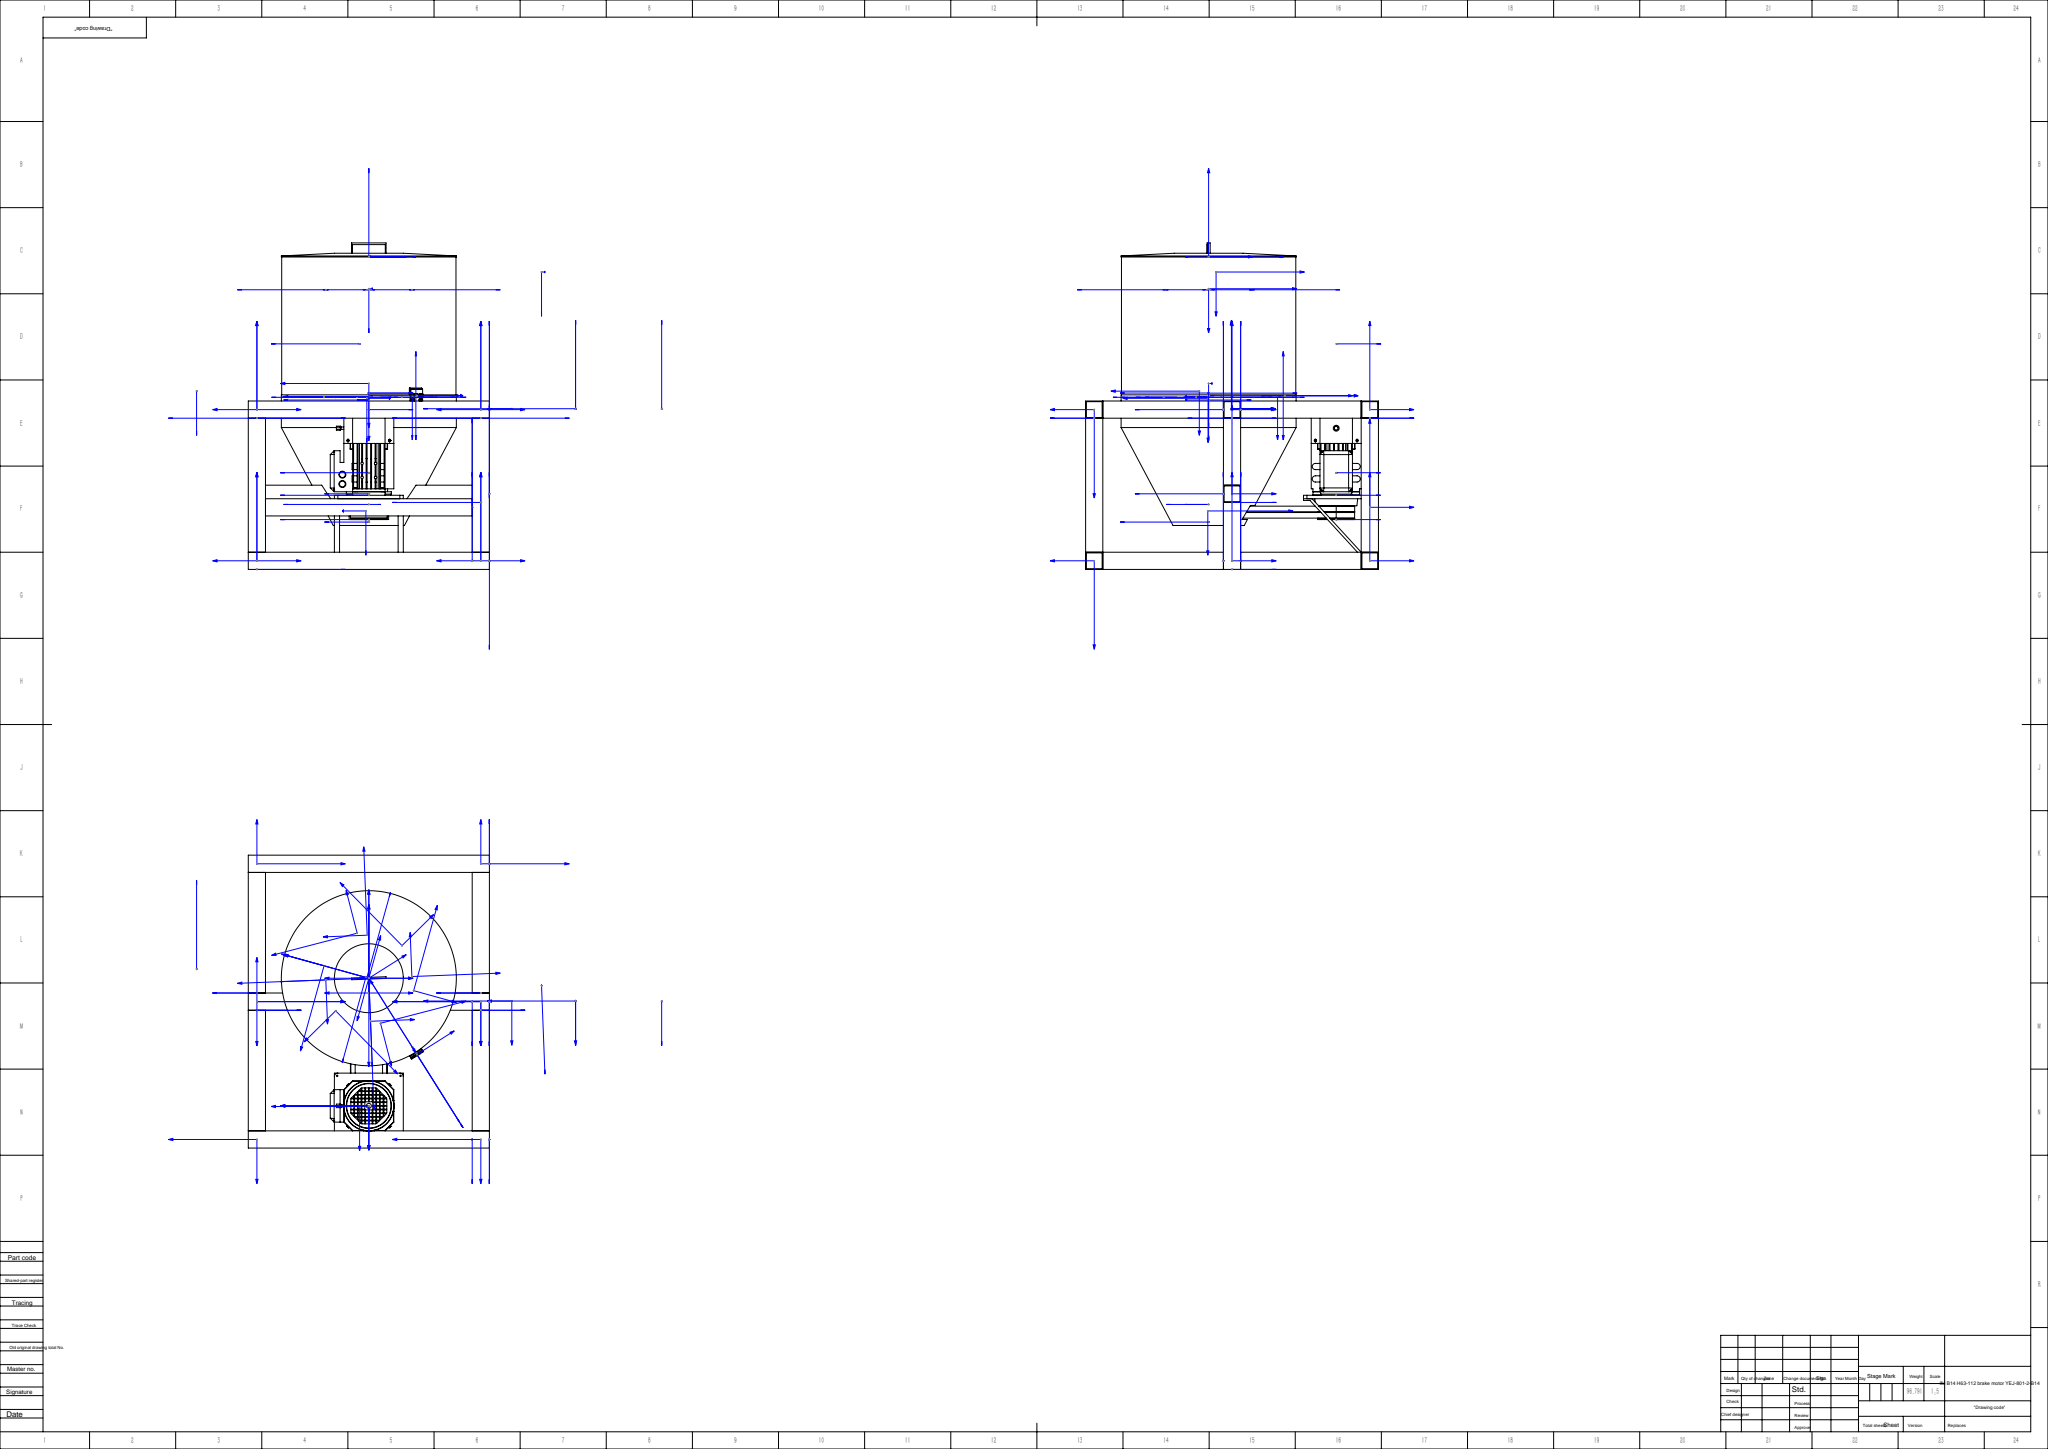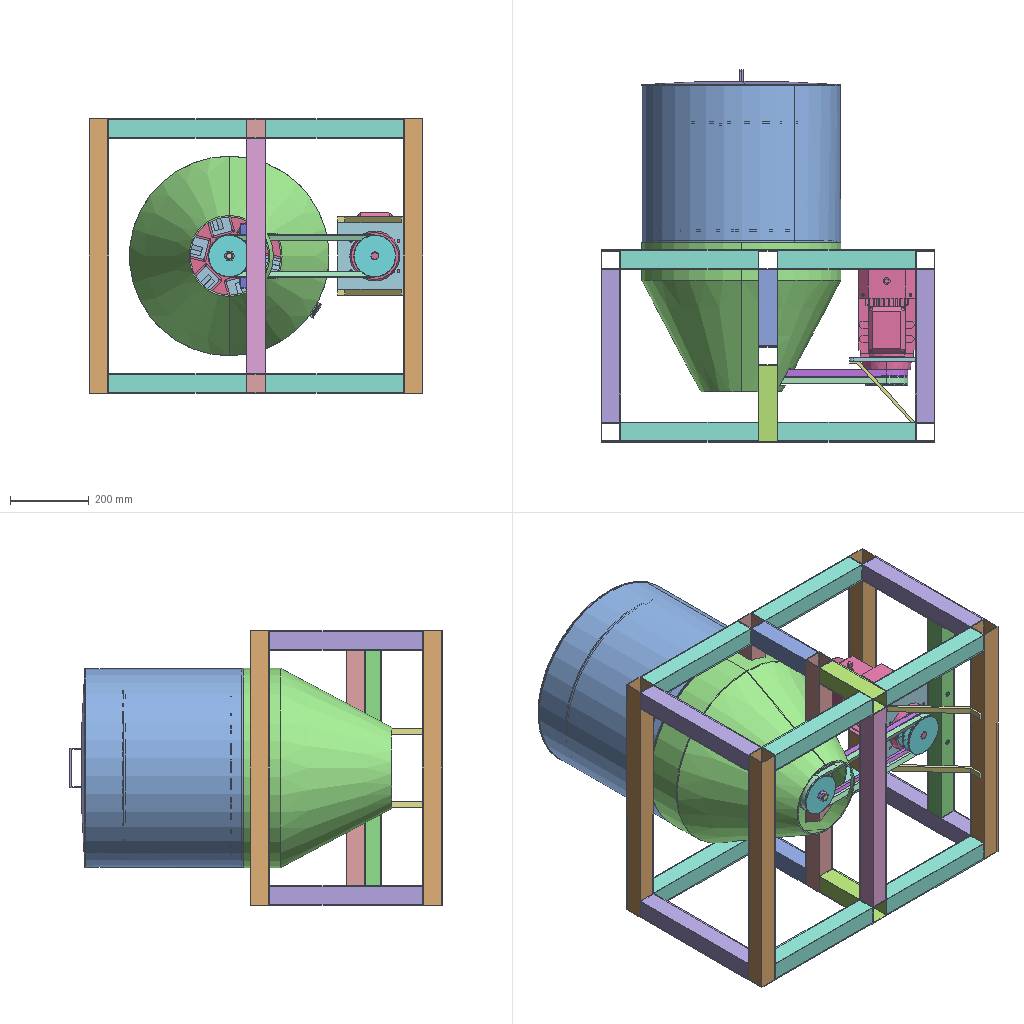Assembly | SolidWorks | 37 different items | 64 placed | box 850 x 948 x 700 mm
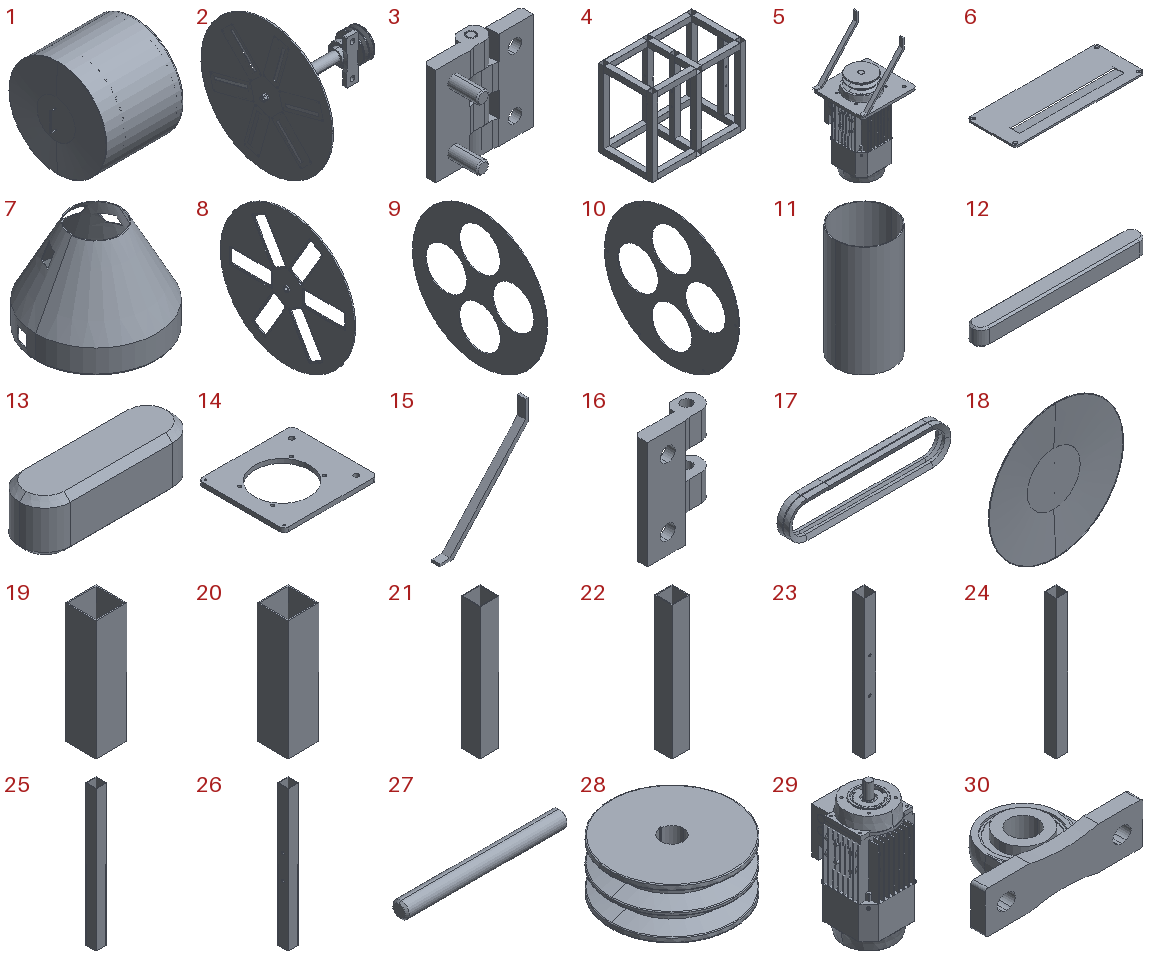Parts list (item | name | quantity | parent item | size | volume | features):
1 | (subassembly) | x1 | - | 463.5 x 508 x 508 mm | 4178464 mm3 | features ReferencePattern 3, LocalCirPattern 1
2 | (subassembly) | x1 | - | 394 x 496 x 496 mm | 1816231 mm3 | features ReferencePattern 5, LocalCirPattern 1
3 | (subassembly) | x1 | in 1 | 40 x 21 x 40 mm | 8853 mm3 | features AEMSimFeature 1
4 | (subassembly) | x1 | - | 850 x 488.8 x 700 mm | 4041372 mm3 | -
5 | (subassembly) | x1 | - | 217.5 x 212 x 474.6 mm | 5596236 mm3 | features CompositeCurve 1, MirrorCompFeat 1, ReferencePattern 1
6 | - | x6 | in 2 | 160 x 60 x 2 mm | 16130 mm3 | features ICE 2, Extrusion 1, Fillet 1, HoleWzd 1
7 | - | x1 | - | 508 x 508 x 384 mm | 1629335 mm3 | features Cut 2, Extrusion 1, ICE 1, Revolution 1
8 | - | x1 | in 2 | 15 x 496 x 496 mm | 717635 mm3 | features ICE 6, CirPattern 2, Fillet 2, Cut 1, Extrusion 1, HoleWzd 1
9 | - | x1 | in 1 | 3 x 500 x 500 mm | 365531 mm3 | features CirPattern 2, ICE 2, Extrusion 1
10 | - | x1 | in 1 | 3 x 500 x 500 mm | 376482 mm3 | features CirPattern 2, ICE 2, Extrusion 1
11 | - | x4 | in 1 | 154 x 154 x 300 mm | 286513 mm3 | features Extrusion 1
12 | - | x1 | in 2 | 20 x 2 x 2 mm | 76.609 mm3 | features BaseBody 1
13 | - | x1 | in 2 | 6 x 2 x 2 mm | 21.423 mm3 | features BaseBody 1
14 | - | x1 | in 5 | 217.5 x 200 x 10 mm | 301745 mm3 | features ICE 3, Cut 2, Extrusion 1, Fillet 1, HoleWzd 1
15 | - | x2 | in 5 | 167.5 x 15 x 195.2 mm | 29797 mm3 | features Extrusion 1
16 | - | x1 | in 3 | 25 x 9 x 40 mm | 3717 mm3 | features BaseBody 1
17 | - | x1 | - | 477.4 x 34.776 x 107 mm | 340043 mm3 | features Sweep 1
18 | - | x1 | in 1 | 508 x 41 x 508 mm | 209061 mm3 | features ICE 1, Revolution 1
19 | - | x2 | in 4 | 50 x 50 x 194.4 mm | 74650 mm3 | features Extrusion 1, ICE 1
20 | - | x2 | in 4 | 50 x 50 x 194.4 mm | 74650 mm3 | features Extrusion 1
21 | - | x8 | in 4 | 50 x 50 x 350 mm | 134400 mm3 | features Extrusion 1
22 | - | x4 | in 4 | 50 x 50 x 388.8 mm | 149299 mm3 | features Extrusion 1
23 | - | x1 | in 4 | 50 x 50 x 600 mm | 229640 mm3 | features Cut 1, Extrusion 1
24 | - | x1 | in 4 | 50 x 50 x 600 mm | 230400 mm3 | features Extrusion 1
25 | - | x4 | in 4 | 50 x 50 x 700 mm | 268800 mm3 | features Extrusion 1
26 | - | x2 | in 4 | 50 x 50 x 700 mm | 267568 mm3 | features Extrusion 1, ICE 1
27 | - | x1 | in 3 | 40 x 4 x 4 mm | 499.775 mm3 | features BaseBody 1
28 | - | x2 | in 2, 5 | 107 x 107 x 44 mm | 283777 mm3 | features ICE 3, BaseBody 1
29 | - | x1 | in 5 | 145.261 x 184.63 x 340 mm | 4951111 mm3 | features BaseBody 1
30 | - | x2 | in 2 | 165 x 83 x 44.2 mm | 207279 mm3 | features BaseBody 4, ICE 1
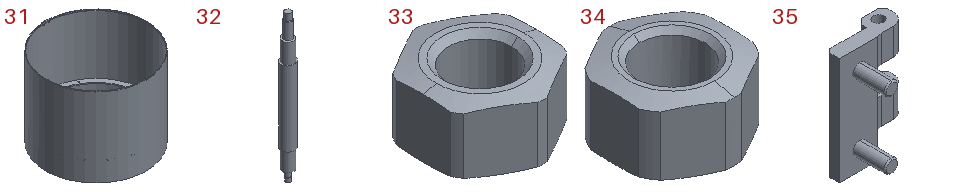31 | - | x1 | in 1 | 506 x 509 x 400 mm | 2072487 mm3 | features ICE 6, CirPattern 1, Extrusion 1
32 | - | x1 | in 2 | 36 x 36 x 394 mm | 296771 mm3 | features ICE 9, Extrusion 1
33 | - | x1 | in 2 | 18 x 20 x 10.5 mm | 1969 mm3 | features BaseBody 1
34 | - | x1 | in 2 | 24 x 26 x 14.5 mm | 4644 mm3 | features BaseBody 1
35 | - | x1 | in 3 | 25 x 21 x 40 mm | 4636 mm3 | features BaseBody 1
36 | GB╱T 70.1-2008[Hex Socket Head Cap Screw M10×80] | x1 | - | - | - | -
37 | Hex Nut Standard[PNHC-M10-B] | x1 | - | - | - | -
Mates (type | each side: item.copy, entity, surface, feature):
In the top assembly
Coincident | 26.1 face plane Boss-Extrude1 | 30.1 face plane Input1
Concentric | 26.1 face cylinder Cut-Extrude1 | 30.1 face cylinder Cut-Extrude1 | 2 times
Concentric | 32.1 face cylinder Boss-Extrude2 | 7.1 face cylinder Boss-Extrude1
DistanceDim | 7.1 face plane Boss-Extrude1 | 8.1 face plane Boss-Extrude1
Concentric | 31.1 face cylinder Boss-Extrude1 | 7.1 face cylinder Boss-Extrude1
Coincident | 31.1 face plane Boss-Extrude1 | 7.1 face plane Cut-Extrude4
Parallel | 25.1 face plane Boss-Extrude1 | 28.1 face plane Input1
Coincident | 28.2 face plane Input1 | 28.1 face plane Input1
Width | 29.1 face plane Input1 | 29.1 face plane Input1 | 22.1 face plane Boss-Extrude1 | 22.2 face plane Boss-Extrude1
Coincident | 25.2 face plane Boss-Extrude1 | 29.1 face plane Input1
In subassembly 2
Coincident | 8.2 face plane Cut-Extrude2 | 6.1 face plane Boss-Extrude1 | 3 times
Coincident | 8.2 face plane Boss-Extrude2 | 32.2 face plane Boss-Extrude1
Concentric | 8.2 face cylinder Cut-Extrude4 | 32.2 face cylinder Boss-Extrude4
Coincident | 32.2 face plane Cut-Extrude1 | 13.1 face plane Input1
Concentric | 32.2 face cylinder Cut-Extrude1 | 13.1 face cylinder Input1 | 2 times
Parallel | 8.2 face plane Cut-Extrude5 | 13.1 face plane Input1
Concentric | 32.2 face cylinder Boss-Extrude4 | 33.1 face cylinder Input1
Coincident | 8.2 face plane Boss-Extrude2 | 33.1 face plane Input1
Concentric | 32.2 face cylinder Boss-Extrude3 | 30.2 face cylinder Input2
Coincident | 32.2 face plane Boss-Extrude2 | 30.2 face plane Input2
Coincident | 32.2 face plane Cut-Extrude4 | 28.3 face plane Cut-Extrude2
Coincident | 32.2 face plane Cut-Extrude4 | 12.1 face plane Input1
Concentric | 32.2 face cylinder Cut-Extrude4 | 12.1 face cylinder Input1 | 2 times
Concentric | 32.2 face cylinder Boss-Extrude5 | 28.3 face cylinder Cut-Extrude1
Coincident | 32.2 face plane Boss-Extrude3 | 28.3 face plane Input1
Concentric | 32.2 face cylinder Boss-Extrude6 | 34.1 face cylinder Input1
Coincident | 28.3 face plane Input1 | 34.1 face plane Input1
Concentric | 32.2 face cylinder Boss-Extrude1 | 30.3 face cylinder Input2
Coincident | 32.2 face plane Boss-Extrude2 | 30.3 face plane Input2
Coincident | 30.3 face plane Input1 | 30.2 face plane Input1
In subassembly 5
Concentric | 29.2 face cylinder Input1 | 28.3 face cylinder Cut-Extrude1
Coincident | 29.2 face plane Input1 | 28.3 face plane Input1
Coincident | 29.2 face plane Input1 | 14.1 face plane Boss-Extrude1
Concentric | 29.2 edge | 14.1 face cylinder Cut-Extrude1
In subassembly 1
Coincident | 10.1 face plane Boss-Extrude1 | 11.1 face plane Boss-Extrude1
Concentric | 10.1 face cylinder Cut-Extrude1 | 11.1 face cylinder Boss-Extrude1
Concentric | 10.1 face cylinder Boss-Extrude1 | 31.2 face cylinder Boss-Extrude1
Coincident | 10.1 face plane Boss-Extrude1 | 31.2 face plane Boss-Extrude2
Concentric | 10.1 face cylinder CirPattern2 | 31.2 face cylinder Cut-Extrude1
Concentric | 11.1 face cylinder Boss-Extrude1 | 9.1 face cylinder CirPattern1
Concentric | 31.2 face cylinder Boss-Extrude1 | 9.1 face cylinder Boss-Extrude1
DistanceDim | 9.1 face plane Boss-Extrude1 | 31.2 face plane Boss-Extrude1
Concentric | 31.2 face cylinder Boss-Extrude1 | 18.1 face cylinder Revolve1
Coincident | 31.2 face plane Boss-Extrude1 | 18.1 face plane Revolve1
Concentric | 31.2 face cylinder Cut-Extrude2 | 35.1 face cylinder Input1
In subassembly 4
Coincident | 26.2 face plane Boss-Extrude1 | 20.1 face plane Boss-Extrude1 | 3 times
Coincident | 26.2 face plane Boss-Extrude1 | 20.2 face plane Boss-Extrude1 | 3 times
Coincident | 20.2 face plane Boss-Extrude1 | 26.3 face plane Boss-Extrude1 | 2 times
Coincident | 26.2 face plane Boss-Extrude1 | 26.3 face plane Boss-Extrude1
Coincident | 26.3 face plane Boss-Extrude1 | 19.1 face plane Boss-Extrude1 | 3 times
Coincident | 26.3 face plane Boss-Extrude1 | 19.2 face plane Boss-Extrude1 | 3 times
Coincident | 19.2 face plane Boss-Extrude1 | 24.1 face plane Boss-Extrude1 | 3 times
Coincident | 26.2 face plane Boss-Extrude1 | 21.1 face plane Boss-Extrude1 | 2 times
Coincident | 20.1 face plane Boss-Extrude1 | 21.1 face plane Boss-Extrude1
Coincident | 26.2 face plane Boss-Extrude1 | 21.2 face plane Boss-Extrude1
Coincident | 21.1 face plane Boss-Extrude1 | 21.2 face plane Boss-Extrude1 | 2 times
Coincident | 26.2 face plane Boss-Extrude1 | 21.3 face plane Boss-Extrude1 | 2 times
Coincident | 20.2 face plane Boss-Extrude1 | 21.3 face plane Boss-Extrude1
Coincident | 26.2 face plane Boss-Extrude1 | 21.4 face plane Boss-Extrude1
Coincident | 19.1 face plane Boss-Extrude1 | 21.4 face plane Boss-Extrude1
Coincident | 24.1 face plane Boss-Extrude1 | 21.4 face plane Boss-Extrude1
Coincident | 26.2 face plane Boss-Extrude1 | 21.5 face plane Boss-Extrude1
Coincident | 19.2 face plane Boss-Extrude1 | 21.5 face plane Boss-Extrude1
Coincident | 24.1 face plane Boss-Extrude1 | 21.5 face plane Boss-Extrude1
Coincident | 26.2 face plane Boss-Extrude1 | 21.6 face plane Boss-Extrude1 | 2 times
Coincident | 20.2 face plane Boss-Extrude1 | 21.6 face plane Boss-Extrude1
Coincident | 26.2 face plane Boss-Extrude1 | 21.7 face plane Boss-Extrude1
Coincident | 19.1 face plane Boss-Extrude1 | 21.7 face plane Boss-Extrude1
Coincident | 24.1 face plane Boss-Extrude1 | 21.7 face plane Boss-Extrude1
Coincident | 26.2 face plane Boss-Extrude1 | 21.8 face plane Boss-Extrude1
Coincident | 19.2 face plane Boss-Extrude1 | 21.8 face plane Boss-Extrude1
Coincident | 24.1 face plane Boss-Extrude1 | 21.8 face plane Boss-Extrude1
Coincident | 21.6 face plane Boss-Extrude1 | 25.3 face plane Boss-Extrude1 | 2 times
Coincident | 21.1 face plane Boss-Extrude1 | 25.3 face plane Boss-Extrude1
Coincident | 21.8 face plane Boss-Extrude1 | 25.4 face plane Boss-Extrude1 | 2 times
Coincident | 21.7 face plane Boss-Extrude1 | 25.4 face plane Boss-Extrude1
Coincident | 21.3 face plane Boss-Extrude1 | 25.5 face plane Boss-Extrude1
Coincident | 21.2 face plane Boss-Extrude1 | 25.5 face plane Boss-Extrude1 | 2 times
Coincident | 21.3 face plane Boss-Extrude1 | 25.6 face plane Boss-Extrude1
Coincident | 21.4 face plane Boss-Extrude1 | 25.6 face plane Boss-Extrude1
Coincident | 21.5 face plane Boss-Extrude1 | 25.6 face plane Boss-Extrude1
Coincident | 25.3 face plane Boss-Extrude1 | 22.3 face plane Boss-Extrude1 | 2 times
Coincident | 21.1 face plane Boss-Extrude1 | 22.3 face plane Boss-Extrude1
Coincident | 25.3 face plane Boss-Extrude1 | 22.4 face plane Boss-Extrude1 | 2 times
Coincident | 21.6 face plane Boss-Extrude1 | 22.4 face plane Boss-Extrude1
Coincident | 25.3 face plane Boss-Extrude1 | 22.5 face plane Boss-Extrude1
Coincident | 25.5 face plane Boss-Extrude1 | 22.5 face plane Boss-Extrude1
Coincident | 21.2 face plane Boss-Extrude1 | 22.5 face plane Boss-Extrude1
Coincident | 25.3 face plane Boss-Extrude1 | 22.6 face plane Boss-Extrude1
Coincident | 25.5 face plane Boss-Extrude1 | 22.6 face plane Boss-Extrude1
Coincident | 21.3 face plane Boss-Extrude1 | 22.6 face plane Boss-Extrude1
Coincident | 22.4 face plane Boss-Extrude1 | 23.1 face plane Boss-Extrude1 | 2 times
DistanceDim | 23.1 face plane Boss-Extrude1 | 25.4 face plane Boss-Extrude1